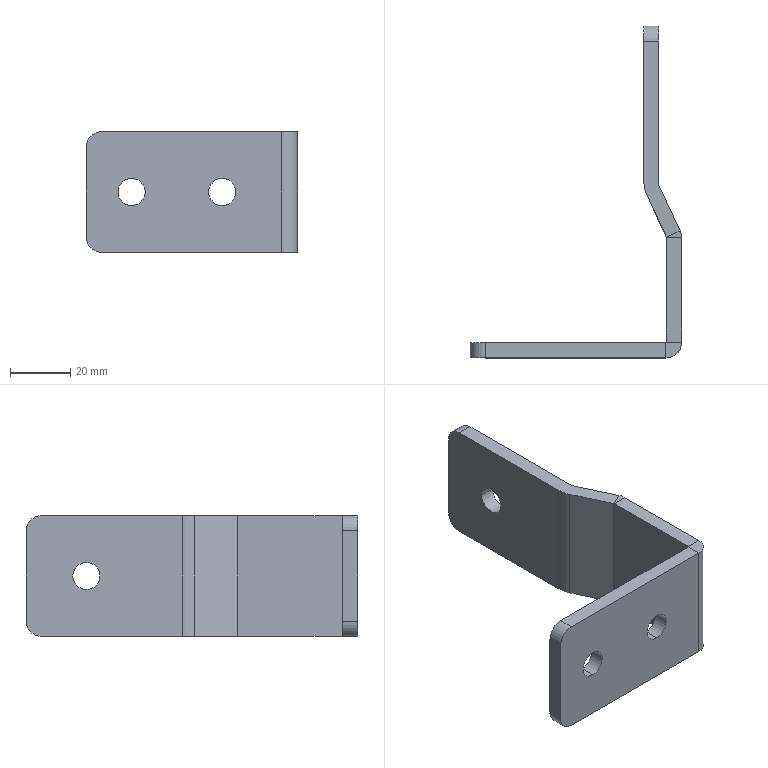Part | SolidWorks | features ICE 3, Fillet 2, MoveFace 2, BaseBody 1 | 1 solid | 340 faces | box 70 x 110 x 40 mm | volume 34015 mm3 | plane 223 | spline 102 | cylinder 15 | commonest cylinder face diameters 9 x6 10 x4 0.4 x2 10.4 x2 20 x1